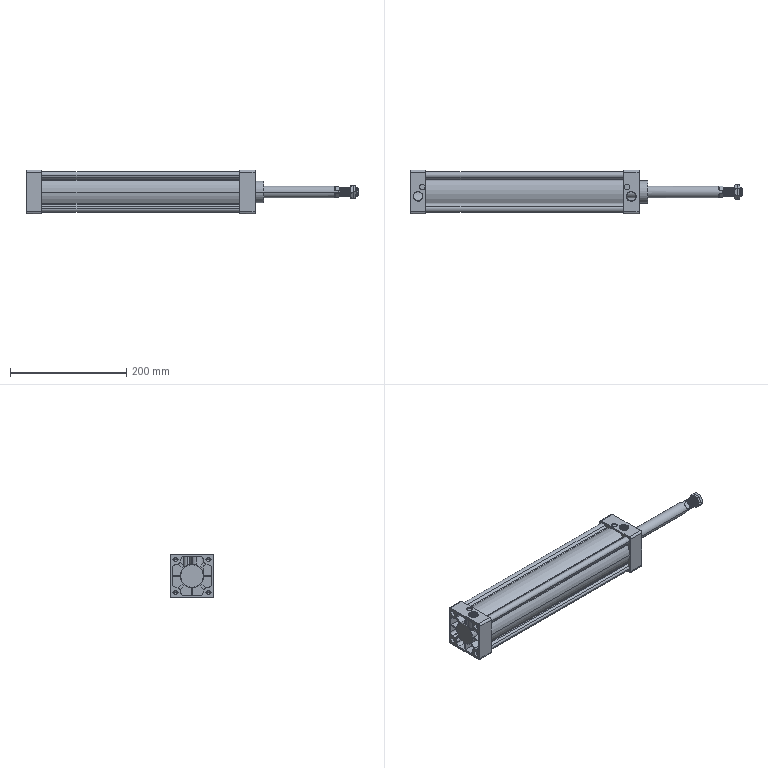Part | STEP file | 102000010555 | 4 solids | 942 faces | box 572.24 x 75 x 75 mm | volume 1547367 mm3 | cylinder 637 | plane 234 | cone 47 | spline 22 | torus 2 | commonest cylinder face diameters 7 x185 8 x177 16 x90 17 x50 14 x41 10 x22